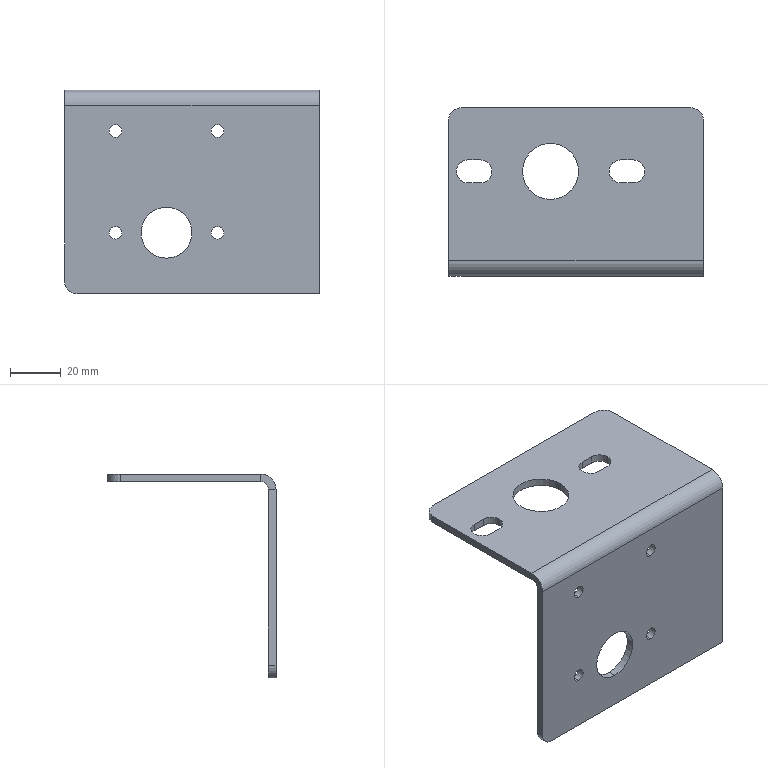Part | SolidWorks | features BaseBody 1 | 1 solid | 39 faces | box 100 x 66 x 80 mm | volume 39302 mm3 | cylinder 23 | plane 16 | commonest cylinder face diameters 5 x8 9 x6 10 x3 20 x2 22 x2 6 x1
STEP:
#1=CARTESIAN_POINT('',(-45.,-34.5,-77.));
#2=VERTEX_POINT('',#1);
#3=CARTESIAN_POINT('',(-50.,-34.5,-72.));
#4=VERTEX_POINT('',#3);
#5=CARTESIAN_POINT('',(-45.,-34.5,-72.));
#6=DIRECTION('',(0.,1.,0.));
#7=DIRECTION('',(0.,0.,1.));
#8=AXIS2_PLACEMENT_3D('',#5,#6,#7);
#9=CIRCLE('',#8,5.);
#10=EDGE_CURVE('',#2,#4,#9,.T.);
#11=ORIENTED_EDGE('',*,*,#10,.T.);
#12=CARTESIAN_POINT('',(-50.,-31.5,-72.));
#13=VERTEX_POINT('',#12);
#14=CARTESIAN_POINT('',(-50.,-34.5,-72.));
#15=DIRECTION('',(0.,1.,0.));
#16=VECTOR('',#15,1000.);
#17=LINE('',#14,#16);
#18=EDGE_CURVE('',#4,#13,#17,.T.);
#19=ORIENTED_EDGE('',*,*,#18,.T.);
#20=CARTESIAN_POINT('',(-45.,-31.5,-77.));
#21=VERTEX_POINT('',#20);
#22=CARTESIAN_POINT('',(-45.,-31.5,-72.));
#23=DIRECTION('',(0.,-1.,0.));
#24=DIRECTION('',(0.,0.,1.));
#25=AXIS2_PLACEMENT_3D('',#22,#23,#24);
#26=CIRCLE('',#25,5.);
#27=EDGE_CURVE('',#13,#21,#26,.T.);
#28=ORIENTED_EDGE('',*,*,#27,.T.);
#29=CARTESIAN_POINT('',(-45.,-34.5,-77.));
#30=DIRECTION('',(0.,-1.,0.));
#31=VECTOR('',#30,1000.);
#32=LINE('',#29,#31);
#33=EDGE_CURVE('',#21,#2,#32,.T.);
#34=ORIENTED_EDGE('',*,*,#33,.T.);
#35=EDGE_LOOP('',(#11,#19,#28,#34));
#36=FACE_OUTER_BOUND('',#35,.T.);
#37=CARTESIAN_POINT('',(-45.,-34.5,-72.));
#38=DIRECTION('',(0.,1.,0.));
#39=DIRECTION('',(0.,0.,-1.));
#40=AXIS2_PLACEMENT_3D('',#37,#38,#39);
#41=CYLINDRICAL_SURFACE('',#40,5.);
#42=ADVANCED_FACE('',(#36),#41,.T.);
#43=CARTESIAN_POINT('',(10.,-34.5,-50.5));
#44=VERTEX_POINT('',#43);
#45=CARTESIAN_POINT('',(10.,-31.5,-50.5));
#46=VERTEX_POINT('',#45);
#47=CARTESIAN_POINT('',(10.,-41.5,-50.5));
#48=DIRECTION('',(0.,1.,0.));
#49=VECTOR('',#48,1000.);
#50=LINE('',#47,#49);
#51=EDGE_CURVE('',#44,#46,#50,.T.);
#52=ORIENTED_EDGE('',*,*,#51,.F.);
#53=CARTESIAN_POINT('',(10.,-34.5,-55.5));
#54=VERTEX_POINT('',#53);
#55=CARTESIAN_POINT('',(10.,-34.5,-53.));
#56=DIRECTION('',(0.,1.,0.));
#57=DIRECTION('',(0.,0.,1.));
#58=AXIS2_PLACEMENT_3D('',#55,#56,#57);
#59=CIRCLE('',#58,2.5);
#60=EDGE_CURVE('',#54,#44,#59,.T.);
#61=ORIENTED_EDGE('',*,*,#60,.F.);
#62=CARTESIAN_POINT('',(10.,-31.5,-55.5));
#63=VERTEX_POINT('',#62);
#64=CARTESIAN_POINT('',(10.,-41.5,-55.5));
#65=DIRECTION('',(0.,1.,0.));
#66=VECTOR('',#65,1000.);
#67=LINE('',#64,#66);
#68=EDGE_CURVE('',#54,#63,#67,.T.);
#69=ORIENTED_EDGE('',*,*,#68,.T.);
#70=CARTESIAN_POINT('',(10.,-31.5,-53.));
#71=DIRECTION('',(0.,-1.,0.));
#72=DIRECTION('',(0.,0.,-1.));
#73=AXIS2_PLACEMENT_3D('',#70,#71,#72);
#74=CIRCLE('',#73,2.5);
#75=EDGE_CURVE('',#46,#63,#74,.T.);
#76=ORIENTED_EDGE('',*,*,#75,.F.);
#77=EDGE_LOOP('',(#52,#61,#69,#76));
#78=FACE_OUTER_BOUND('',#77,.T.);
#79=CARTESIAN_POINT('',(10.,-41.5,-53.));
#80=DIRECTION('',(0.,1.,0.));
#81=DIRECTION('',(0.,0.,-1.));
#82=AXIS2_PLACEMENT_3D('',#79,#80,#81);
#83=CYLINDRICAL_SURFACE('',#82,2.5);
#84=ADVANCED_FACE('',(#78),#83,.F.);
#85=CARTESIAN_POINT('',(10.,-34.5,-10.5));
#86=VERTEX_POINT('',#85);
#87=CARTESIAN_POINT('',(10.,-31.5,-10.5));
#88=VERTEX_POINT('',#87);
#89=CARTESIAN_POINT('',(10.,-41.5,-10.5));
#90=DIRECTION('',(0.,1.,0.));
#91=VECTOR('',#90,1000.);
#92=LINE('',#89,#91);
#93=EDGE_CURVE('',#86,#88,#92,.T.);
#94=ORIENTED_EDGE('',*,*,#93,.F.);
#95=CARTESIAN_POINT('',(10.,-34.5,-15.5));
#96=VERTEX_POINT('',#95);
#97=CARTESIAN_POINT('',(10.,-34.5,-13.));
#98=DIRECTION('',(0.,1.,0.));
#99=DIRECTION('',(0.,0.,1.));
#100=AXIS2_PLACEMENT_3D('',#97,#98,#99);
#101=CIRCLE('',#100,2.5);
#102=EDGE_CURVE('',#96,#86,#101,.T.);
#103=ORIENTED_EDGE('',*,*,#102,.F.);
#104=CARTESIAN_POINT('',(10.,-31.5,-15.5));
#105=VERTEX_POINT('',#104);
#106=CARTESIAN_POINT('',(10.,-41.5,-15.5));
#107=DIRECTION('',(0.,1.,0.));
#108=VECTOR('',#107,1000.);
#109=LINE('',#106,#108);
#110=EDGE_CURVE('',#96,#105,#109,.T.);
#111=ORIENTED_EDGE('',*,*,#110,.T.);
#112=CARTESIAN_POINT('',(10.,-31.5,-13.));
#113=DIRECTION('',(0.,-1.,0.));
#114=DIRECTION('',(0.,0.,-1.));
#115=AXIS2_PLACEMENT_3D('',#112,#113,#114);
#116=CIRCLE('',#115,2.5);
#117=EDGE_CURVE('',#88,#105,#116,.T.);
#118=ORIENTED_EDGE('',*,*,#117,.F.);
#119=EDGE_LOOP('',(#94,#103,#111,#118));
#120=FACE_OUTER_BOUND('',#119,.T.);
#121=CARTESIAN_POINT('',(10.,-41.5,-13.));
#122=DIRECTION('',(0.,1.,0.));
#123=DIRECTION('',(0.,0.,-1.));
#124=AXIS2_PLACEMENT_3D('',#121,#122,#123);
#125=CYLINDRICAL_SURFACE('',#124,2.5);
#126=ADVANCED_FACE('',(#120),#125,.F.);
#127=CARTESIAN_POINT('',(-30.,-34.5,-10.5));
#128=VERTEX_POINT('',#127);
#129=CARTESIAN_POINT('',(-30.,-31.5,-10.5));
#130=VERTEX_POINT('',#129);
#131=CARTESIAN_POINT('',(-30.,-41.5,-10.5));
#132=DIRECTION('',(0.,1.,0.));
#133=VECTOR('',#132,1000.);
#134=LINE('',#131,#133);
#135=EDGE_CURVE('',#128,#130,#134,.T.);
#136=ORIENTED_EDGE('',*,*,#135,.F.);
#137=CARTESIAN_POINT('',(-30.,-34.5,-15.5));
#138=VERTEX_POINT('',#137);
#139=CARTESIAN_POINT('',(-30.,-34.5,-13.));
#140=DIRECTION('',(0.,1.,0.));
#141=DIRECTION('',(0.,0.,1.));
#142=AXIS2_PLACEMENT_3D('',#139,#140,#141);
#143=CIRCLE('',#142,2.5);
#144=EDGE_CURVE('',#138,#128,#143,.T.);
#145=ORIENTED_EDGE('',*,*,#144,.F.);
#146=CARTESIAN_POINT('',(-30.,-31.5,-15.5));
#147=VERTEX_POINT('',#146);
#148=CARTESIAN_POINT('',(-30.,-41.5,-15.5));
#149=DIRECTION('',(0.,1.,0.));
#150=VECTOR('',#149,1000.);
#151=LINE('',#148,#150);
#152=EDGE_CURVE('',#138,#147,#151,.T.);
#153=ORIENTED_EDGE('',*,*,#152,.T.);
#154=CARTESIAN_POINT('',(-30.,-31.5,-13.));
#155=DIRECTION('',(0.,-1.,0.));
#156=DIRECTION('',(0.,0.,-1.));
#157=AXIS2_PLACEMENT_3D('',#154,#155,#156);
#158=CIRCLE('',#157,2.5);
#159=EDGE_CURVE('',#130,#147,#158,.T.);
#160=ORIENTED_EDGE('',*,*,#159,.F.);
#161=EDGE_LOOP('',(#136,#145,#153,#160));
#162=FACE_OUTER_BOUND('',#161,.T.);
#163=CARTESIAN_POINT('',(-30.,-41.5,-13.));
#164=DIRECTION('',(0.,1.,0.));
#165=DIRECTION('',(0.,0.,-1.));
#166=AXIS2_PLACEMENT_3D('',#163,#164,#165);
#167=CYLINDRICAL_SURFACE('',#166,2.5);
#168=ADVANCED_FACE('',(#162),#167,.F.);
#169=CARTESIAN_POINT('',(-30.,-34.5,-50.5));
#170=VERTEX_POINT('',#169);
#171=CARTESIAN_POINT('',(-30.,-31.5,-50.5));
#172=VERTEX_POINT('',#171);
#173=CARTESIAN_POINT('',(-30.,-41.5,-50.5));
#174=DIRECTION('',(0.,1.,0.));
#175=VECTOR('',#174,1000.);
#176=LINE('',#173,#175);
#177=EDGE_CURVE('',#170,#172,#176,.T.);
#178=ORIENTED_EDGE('',*,*,#177,.F.);
#179=CARTESIAN_POINT('',(-30.,-34.5,-55.5));
#180=VERTEX_POINT('',#179);
#181=CARTESIAN_POINT('',(-30.,-34.5,-53.));
#182=DIRECTION('',(0.,1.,0.));
#183=DIRECTION('',(0.,0.,1.));
#184=AXIS2_PLACEMENT_3D('',#181,#182,#183);
#185=CIRCLE('',#184,2.5);
#186=EDGE_CURVE('',#180,#170,#185,.T.);
#187=ORIENTED_EDGE('',*,*,#186,.F.);
#188=CARTESIAN_POINT('',(-30.,-31.5,-55.5));
#189=VERTEX_POINT('',#188);
#190=CARTESIAN_POINT('',(-30.,-41.5,-55.5));
#191=DIRECTION('',(0.,1.,0.));
#192=VECTOR('',#191,1000.);
#193=LINE('',#190,#192);
#194=EDGE_CURVE('',#180,#189,#193,.T.);
#195=ORIENTED_EDGE('',*,*,#194,.T.);
#196=CARTESIAN_POINT('',(-30.,-31.5,-53.));
#197=DIRECTION('',(0.,-1.,0.));
#198=DIRECTION('',(0.,0.,-1.));
#199=AXIS2_PLACEMENT_3D('',#196,#197,#198);
#200=CIRCLE('',#199,2.5);
#201=EDGE_CURVE('',#172,#189,#200,.T.);
#202=ORIENTED_EDGE('',*,*,#201,.F.);
#203=EDGE_LOOP('',(#178,#187,#195,#202));
#204=FACE_OUTER_BOUND('',#203,.T.);
#205=CARTESIAN_POINT('',(-30.,-41.5,-53.));
#206=DIRECTION('',(0.,1.,0.));
#207=DIRECTION('',(0.,0.,-1.));
#208=AXIS2_PLACEMENT_3D('',#205,#206,#207);
#209=CYLINDRICAL_SURFACE('',#208,2.5);
#210=ADVANCED_FACE('',(#204),#209,.F.);
#211=CARTESIAN_POINT('',(-10.,-34.5,-43.));
#212=VERTEX_POINT('',#211);
#213=CARTESIAN_POINT('',(-10.,-31.5,-43.));
#214=VERTEX_POINT('',#213);
#215=CARTESIAN_POINT('',(-10.,-41.5,-43.));
#216=DIRECTION('',(0.,1.,0.));
#217=VECTOR('',#216,1000.);
#218=LINE('',#215,#217);
#219=EDGE_CURVE('',#212,#214,#218,.T.);
#220=ORIENTED_EDGE('',*,*,#219,.F.);
#221=CARTESIAN_POINT('',(-10.,-34.5,-63.));
#222=VERTEX_POINT('',#221);
#223=CARTESIAN_POINT('',(-10.,-34.5,-53.));
#224=DIRECTION('',(0.,1.,0.));
#225=DIRECTION('',(0.,0.,1.));
#226=AXIS2_PLACEMENT_3D('',#223,#224,#225);
#227=CIRCLE('',#226,10.);
#228=EDGE_CURVE('',#222,#212,#227,.T.);
#229=ORIENTED_EDGE('',*,*,#228,.F.);
#230=CARTESIAN_POINT('',(-10.,-31.5,-63.));
#231=VERTEX_POINT('',#230);
#232=CARTESIAN_POINT('',(-10.,-41.5,-63.));
#233=DIRECTION('',(0.,1.,0.));
#234=VECTOR('',#233,1000.);
#235=LINE('',#232,#234);
#236=EDGE_CURVE('',#222,#231,#235,.T.);
#237=ORIENTED_EDGE('',*,*,#236,.T.);
#238=CARTESIAN_POINT('',(-10.,-31.5,-53.));
#239=DIRECTION('',(0.,-1.,0.));
#240=DIRECTION('',(0.,0.,-1.));
#241=AXIS2_PLACEMENT_3D('',#238,#239,#240);
#242=CIRCLE('',#241,10.);
#243=EDGE_CURVE('',#214,#231,#242,.T.);
#244=ORIENTED_EDGE('',*,*,#243,.F.);
#245=EDGE_LOOP('',(#220,#229,#237,#244));
#246=FACE_OUTER_BOUND('',#245,.T.);
#247=CARTESIAN_POINT('',(-10.,-41.5,-53.));
#248=DIRECTION('',(0.,1.,0.));
#249=DIRECTION('',(0.,0.,-1.));
#250=AXIS2_PLACEMENT_3D('',#247,#248,#249);
#251=CYLINDRICAL_SURFACE('',#250,10.);
#252=ADVANCED_FACE('',(#246),#251,.F.);
#253=CARTESIAN_POINT('',(-50.,26.5,3.));
#254=VERTEX_POINT('',#253);
#255=CARTESIAN_POINT('',(-45.,31.5,3.));
#256=VERTEX_POINT('',#255);
#257=CARTESIAN_POINT('',(-45.,26.5,3.));
#258=DIRECTION('',(0.,0.,-1.));
#259=DIRECTION('',(1.,0.,0.));
#260=AXIS2_PLACEMENT_3D('',#257,#258,#259);
#261=CIRCLE('',#260,5.);
#262=EDGE_CURVE('',#254,#256,#261,.T.);
#263=ORIENTED_EDGE('',*,*,#262,.T.);
#264=CARTESIAN_POINT('',(-45.,31.5,0.));
#265=VERTEX_POINT('',#264);
#266=CARTESIAN_POINT('',(-45.,31.5,3.));
#267=DIRECTION('',(0.,0.,-1.));
#268=VECTOR('',#267,1000.);
#269=LINE('',#266,#268);
#270=EDGE_CURVE('',#256,#265,#269,.T.);
#271=ORIENTED_EDGE('',*,*,#270,.T.);
#272=CARTESIAN_POINT('',(-50.,26.5,0.));
#273=VERTEX_POINT('',#272);
#274=CARTESIAN_POINT('',(-45.,26.5,0.));
#275=DIRECTION('',(0.,0.,1.));
#276=DIRECTION('',(1.,0.,0.));
#277=AXIS2_PLACEMENT_3D('',#274,#275,#276);
#278=CIRCLE('',#277,5.);
#279=EDGE_CURVE('',#265,#273,#278,.T.);
#280=ORIENTED_EDGE('',*,*,#279,.T.);
#281=CARTESIAN_POINT('',(-50.,26.5,3.));
#282=DIRECTION('',(0.,0.,1.));
#283=VECTOR('',#282,1000.);
#284=LINE('',#281,#283);
#285=EDGE_CURVE('',#273,#254,#284,.T.);
#286=ORIENTED_EDGE('',*,*,#285,.T.);
#287=EDGE_LOOP('',(#263,#271,#280,#286));
#288=FACE_OUTER_BOUND('',#287,.T.);
#289=CARTESIAN_POINT('',(-45.,26.5,3.));
#290=DIRECTION('',(0.,0.,-1.));
#291=DIRECTION('',(1.,0.,0.));
#292=AXIS2_PLACEMENT_3D('',#289,#290,#291);
#293=CYLINDRICAL_SURFACE('',#292,5.);
#294=ADVANCED_FACE('',(#288),#293,.T.);
#295=CARTESIAN_POINT('',(45.,31.5,3.));
#296=VERTEX_POINT('',#295);
#297=CARTESIAN_POINT('',(50.,26.5,3.));
#298=VERTEX_POINT('',#297);
#299=CARTESIAN_POINT('',(45.,26.5,3.));
#300=DIRECTION('',(0.,0.,-1.));
#301=DIRECTION('',(1.,0.,0.));
#302=AXIS2_PLACEMENT_3D('',#299,#300,#301);
#303=CIRCLE('',#302,5.);
#304=EDGE_CURVE('',#296,#298,#303,.T.);
#305=ORIENTED_EDGE('',*,*,#304,.T.);
#306=CARTESIAN_POINT('',(50.,26.5,0.));
#307=VERTEX_POINT('',#306);
#308=CARTESIAN_POINT('',(50.,26.5,3.));
#309=DIRECTION('',(0.,0.,-1.));
#310=VECTOR('',#309,1000.);
#311=LINE('',#308,#310);
#312=EDGE_CURVE('',#298,#307,#311,.T.);
#313=ORIENTED_EDGE('',*,*,#312,.T.);
#314=CARTESIAN_POINT('',(45.,31.5,0.));
#315=VERTEX_POINT('',#314);
#316=CARTESIAN_POINT('',(45.,26.5,0.));
#317=DIRECTION('',(0.,0.,1.));
#318=DIRECTION('',(1.,0.,0.));
#319=AXIS2_PLACEMENT_3D('',#316,#317,#318);
#320=CIRCLE('',#319,5.);
#321=EDGE_CURVE('',#307,#315,#320,.T.);
#322=ORIENTED_EDGE('',*,*,#321,.T.);
#323=CARTESIAN_POINT('',(45.,31.5,3.));
#324=DIRECTION('',(0.,0.,1.));
#325=VECTOR('',#324,1000.);
#326=LINE('',#323,#325);
#327=EDGE_CURVE('',#315,#296,#326,.T.);
#328=ORIENTED_EDGE('',*,*,#327,.T.);
#329=EDGE_LOOP('',(#305,#313,#322,#328));
#330=FACE_OUTER_BOUND('',#329,.T.);
#331=CARTESIAN_POINT('',(45.,26.5,3.));
#332=DIRECTION('',(0.,0.,-1.));
#333=DIRECTION('',(1.,0.,0.));
#334=AXIS2_PLACEMENT_3D('',#331,#332,#333);
#335=CYLINDRICAL_SURFACE('',#334,5.);
#336=ADVANCED_FACE('',(#330),#335,.T.);
#337=CARTESIAN_POINT('',(50.,-31.5,-77.));
#338=VERTEX_POINT('',#337);
#339=CARTESIAN_POINT('',(50.,-31.5,-77.));
#340=DIRECTION('',(1.,0.,0.));
#341=VECTOR('',#340,1000.);
#342=LINE('',#339,#341);
#343=EDGE_CURVE('',#21,#338,#342,.T.);
#344=ORIENTED_EDGE('',*,*,#343,.T.);
#345=CARTESIAN_POINT('',(50.,-34.5,-77.));
#346=VERTEX_POINT('',#345);
#347=CARTESIAN_POINT('',(50.,-34.5,-77.));
#348=DIRECTION('',(0.,1.,0.));
#349=VECTOR('',#348,1000.);
#350=LINE('',#347,#349);
#351=EDGE_CURVE('',#346,#338,#350,.T.);
#352=ORIENTED_EDGE('',*,*,#351,.F.);
#353=CARTESIAN_POINT('',(50.,-34.5,-77.));
#354=DIRECTION('',(1.,0.,0.));
#355=VECTOR('',#354,1000.);
#356=LINE('',#353,#355);
#357=EDGE_CURVE('',#2,#346,#356,.T.);
#358=ORIENTED_EDGE('',*,*,#357,.F.);
#359=ORIENTED_EDGE('',*,*,#33,.F.);
#360=EDGE_LOOP('',(#344,#352,#358,#359));
#361=FACE_OUTER_BOUND('',#360,.T.);
#362=CARTESIAN_POINT('',(50.,-34.5,-77.));
#363=DIRECTION('',(0.,0.,-1.));
#364=DIRECTION('',(0.,-1.,0.));
#365=AXIS2_PLACEMENT_3D('',#362,#363,#364);
#366=PLANE('',#365);
#367=ADVANCED_FACE('',(#361),#366,.T.);
#368=CARTESIAN_POINT('',(-10.,-31.5,-53.));
#369=DIRECTION('',(0.,-1.,0.));
#370=DIRECTION('',(0.,0.,-1.));
#371=AXIS2_PLACEMENT_3D('',#368,#369,#370);
#372=CIRCLE('',#371,10.);
#373=EDGE_CURVE('',#231,#214,#372,.T.);
#374=ORIENTED_EDGE('',*,*,#373,.T.);
#375=ORIENTED_EDGE('',*,*,#243,.T.);
#376=EDGE_LOOP('',(#374,#375));
#377=FACE_BOUND('',#376,.T.);
#378=CARTESIAN_POINT('',(-30.,-31.5,-53.));
#379=DIRECTION('',(0.,-1.,0.));
#380=DIRECTION('',(0.,0.,-1.));
#381=AXIS2_PLACEMENT_3D('',#378,#379,#380);
#382=CIRCLE('',#381,2.5);
#383=EDGE_CURVE('',#189,#172,#382,.T.);
#384=ORIENTED_EDGE('',*,*,#383,.T.);
#385=ORIENTED_EDGE('',*,*,#201,.T.);
#386=EDGE_LOOP('',(#384,#385));
#387=FACE_BOUND('',#386,.T.);
#388=CARTESIAN_POINT('',(-30.,-31.5,-13.));
#389=DIRECTION('',(0.,-1.,0.));
#390=DIRECTION('',(0.,0.,-1.));
#391=AXIS2_PLACEMENT_3D('',#388,#389,#390);
#392=CIRCLE('',#391,2.5);
#393=EDGE_CURVE('',#147,#130,#392,.T.);
#394=ORIENTED_EDGE('',*,*,#393,.T.);
#395=ORIENTED_EDGE('',*,*,#159,.T.);
#396=EDGE_LOOP('',(#394,#395));
#397=FACE_BOUND('',#396,.T.);
#398=CARTESIAN_POINT('',(10.,-31.5,-13.));
#399=DIRECTION('',(0.,-1.,0.));
#400=DIRECTION('',(0.,0.,-1.));
#401=AXIS2_PLACEMENT_3D('',#398,#399,#400);
#402=CIRCLE('',#401,2.5);
#403=EDGE_CURVE('',#105,#88,#402,.T.);
#404=ORIENTED_EDGE('',*,*,#403,.T.);
#405=ORIENTED_EDGE('',*,*,#117,.T.);
#406=EDGE_LOOP('',(#404,#405));
#407=FACE_BOUND('',#406,.T.);
#408=CARTESIAN_POINT('',(10.,-31.5,-53.));
#409=DIRECTION('',(0.,-1.,0.));
#410=DIRECTION('',(0.,0.,-1.));
#411=AXIS2_PLACEMENT_3D('',#408,#409,#410);
#412=CIRCLE('',#411,2.5);
#413=EDGE_CURVE('',#63,#46,#412,.T.);
#414=ORIENTED_EDGE('',*,*,#413,.T.);
#415=ORIENTED_EDGE('',*,*,#75,.T.);
#416=EDGE_LOOP('',(#414,#415));
#417=FACE_BOUND('',#416,.T.);
#418=CARTESIAN_POINT('',(-50.,-31.5,-3.));
#419=VERTEX_POINT('',#418);
#420=CARTESIAN_POINT('',(-50.,-31.5,-77.));
#421=DIRECTION('',(0.,0.,-1.));
#422=VECTOR('',#421,1000.);
#423=LINE('',#420,#422);
#424=EDGE_CURVE('',#419,#13,#423,.T.);
#425=ORIENTED_EDGE('',*,*,#424,.F.);
#426=CARTESIAN_POINT('',(50.,-31.5,-3.));
#427=VERTEX_POINT('',#426);
#428=CARTESIAN_POINT('',(-50.,-31.5,-3.));
#429=DIRECTION('',(1.,0.,0.));
#430=VECTOR('',#429,1000.);
#431=LINE('',#428,#430);
#432=EDGE_CURVE('',#419,#427,#431,.T.);
#433=ORIENTED_EDGE('',*,*,#432,.T.);
#434=CARTESIAN_POINT('',(50.,-31.5,0.));
#435=DIRECTION('',(0.,0.,1.));
#436=VECTOR('',#435,1000.);
#437=LINE('',#434,#436);
#438=EDGE_CURVE('',#338,#427,#437,.T.);
#439=ORIENTED_EDGE('',*,*,#438,.F.);
#440=ORIENTED_EDGE('',*,*,#343,.F.);
#441=ORIENTED_EDGE('',*,*,#27,.F.);
#442=EDGE_LOOP('',(#425,#433,#439,#440,#441));
#443=FACE_OUTER_BOUND('',#442,.T.);
#444=CARTESIAN_POINT('',(0.,-31.5,0.));
#445=DIRECTION('',(0.,-1.,0.));
#446=DIRECTION('',(-1.,0.,0.));
#447=AXIS2_PLACEMENT_3D('',#444,#445,#446);
#448=PLANE('',#447);
#449=ADVANCED_FACE('',(#377,#387,#397,#407,#417,#443),#448,.F.);
#450=ORIENTED_EDGE('',*,*,#228,.T.);
#451=CARTESIAN_POINT('',(-10.,-34.5,-53.));
#452=DIRECTION('',(0.,1.,0.));
#453=DIRECTION('',(0.,0.,1.));
#454=AXIS2_PLACEMENT_3D('',#451,#452,#453);
#455=CIRCLE('',#454,10.);
#456=EDGE_CURVE('',#212,#222,#455,.T.);
#457=ORIENTED_EDGE('',*,*,#456,.T.);
#458=EDGE_LOOP('',(#450,#457));
#459=FACE_BOUND('',#458,.T.);
#460=ORIENTED_EDGE('',*,*,#186,.T.);
#461=CARTESIAN_POINT('',(-30.,-34.5,-53.));
#462=DIRECTION('',(0.,1.,0.));
#463=DIRECTION('',(0.,0.,1.));
#464=AXIS2_PLACEMENT_3D('',#461,#462,#463);
#465=CIRCLE('',#464,2.5);
#466=EDGE_CURVE('',#170,#180,#465,.T.);
#467=ORIENTED_EDGE('',*,*,#466,.T.);
#468=EDGE_LOOP('',(#460,#467));
#469=FACE_BOUND('',#468,.T.);
#470=ORIENTED_EDGE('',*,*,#144,.T.);
#471=CARTESIAN_POINT('',(-30.,-34.5,-13.));
#472=DIRECTION('',(0.,1.,0.));
#473=DIRECTION('',(0.,0.,1.));
#474=AXIS2_PLACEMENT_3D('',#471,#472,#473);
#475=CIRCLE('',#474,2.5);
#476=EDGE_CURVE('',#128,#138,#475,.T.);
#477=ORIENTED_EDGE('',*,*,#476,.T.);
#478=EDGE_LOOP('',(#470,#477));
#479=FACE_BOUND('',#478,.T.);
#480=ORIENTED_EDGE('',*,*,#102,.T.);
#481=CARTESIAN_POINT('',(10.,-34.5,-13.));
#482=DIRECTION('',(0.,1.,0.));
#483=DIRECTION('',(0.,0.,1.));
#484=AXIS2_PLACEMENT_3D('',#481,#482,#483);
#485=CIRCLE('',#484,2.5);
#486=EDGE_CURVE('',#86,#96,#485,.T.);
#487=ORIENTED_EDGE('',*,*,#486,.T.);
#488=EDGE_LOOP('',(#480,#487));
#489=FACE_BOUND('',#488,.T.);
#490=ORIENTED_EDGE('',*,*,#60,.T.);
#491=CARTESIAN_POINT('',(10.,-34.5,-53.));
#492=DIRECTION('',(0.,1.,0.));
#493=DIRECTION('',(0.,0.,1.));
#494=AXIS2_PLACEMENT_3D('',#491,#492,#493);
#495=CIRCLE('',#494,2.5);
#496=EDGE_CURVE('',#44,#54,#495,.T.);
#497=ORIENTED_EDGE('',*,*,#496,.T.);
#498=EDGE_LOOP('',(#490,#497));
#499=FACE_BOUND('',#498,.T.);
#500=ORIENTED_EDGE('',*,*,#357,.T.);
#501=CARTESIAN_POINT('',(50.,-34.5,-3.));
#502=VERTEX_POINT('',#501);
#503=CARTESIAN_POINT('',(50.,-34.5,0.));
#504=DIRECTION('',(0.,0.,1.));
#505=VECTOR('',#504,1000.);
#506=LINE('',#503,#505);
#507=EDGE_CURVE('',#346,#502,#506,.T.);
#508=ORIENTED_EDGE('',*,*,#507,.T.);
#509=CARTESIAN_POINT('',(-50.,-34.5,-3.));
#510=VERTEX_POINT('',#509);
#511=CARTESIAN_POINT('',(0.,-34.5,-3.));
#512=DIRECTION('',(1.,0.,0.));
#513=VECTOR('',#512,1000.);
#514=LINE('',#511,#513);
#515=EDGE_CURVE('',#510,#502,#514,.T.);
#516=ORIENTED_EDGE('',*,*,#515,.F.);
#517=CARTESIAN_POINT('',(-50.,-34.5,-77.));
#518=DIRECTION('',(0.,0.,-1.));
#519=VECTOR('',#518,1000.);
#520=LINE('',#517,#519);
#521=EDGE_CURVE('',#510,#4,#520,.T.);
#522=ORIENTED_EDGE('',*,*,#521,.T.);
#523=ORIENTED_EDGE('',*,*,#10,.F.);
#524=EDGE_LOOP('',(#500,#508,#516,#522,#523));
#525=FACE_OUTER_BOUND('',#524,.T.);
#526=CARTESIAN_POINT('',(0.,-34.5,0.));
#527=DIRECTION('',(0.,-1.,0.));
#528=DIRECTION('',(-1.,0.,0.));
#529=AXIS2_PLACEMENT_3D('',#526,#527,#528);
#530=PLANE('',#529);
#531=ADVANCED_FACE('',(#459,#469,#479,#489,#499,#525),#530,.T.);
#532=ORIENTED_EDGE('',*,*,#521,.F.);
#533=CARTESIAN_POINT('',(-50.,-31.5,-3.));
#534=DIRECTION('',(0.,-1.,0.));
#535=VECTOR('',#534,1000.);
#536=LINE('',#533,#535);
#537=EDGE_CURVE('',#419,#510,#536,.T.);
#538=ORIENTED_EDGE('',*,*,#537,.F.);
#539=ORIENTED_EDGE('',*,*,#424,.T.);
#540=ORIENTED_EDGE('',*,*,#18,.F.);
#541=EDGE_LOOP('',(#532,#538,#539,#540));
#542=FACE_OUTER_BOUND('',#541,.T.);
#543=CARTESIAN_POINT('',(-50.,-34.5,-77.));
#544=DIRECTION('',(-1.,0.,0.));
#545=DIRECTION('',(0.,0.,1.));
#546=AXIS2_PLACEMENT_3D('',#543,#544,#545);
#547=PLANE('',#546);
#548=ADVANCED_FACE('',(#542),#547,.T.);
#549=ORIENTED_EDGE('',*,*,#507,.F.);
#550=ORIENTED_EDGE('',*,*,#351,.T.);
#551=ORIENTED_EDGE('',*,*,#438,.T.);
#552=CARTESIAN_POINT('',(50.,-31.5,-3.));
#553=DIRECTION('',(0.,-1.,0.));
#554=VECTOR('',#553,1000.);
#555=LINE('',#552,#554);
#556=EDGE_CURVE('',#427,#502,#555,.T.);
#557=ORIENTED_EDGE('',*,*,#556,.T.);
#558=EDGE_LOOP('',(#549,#550,#551,#557));
#559=FACE_OUTER_BOUND('',#558,.T.);
#560=CARTESIAN_POINT('',(50.,-34.5,0.));
#561=DIRECTION('',(1.,0.,0.));
#562=DIRECTION('',(0.,1.,0.));
#563=AXIS2_PLACEMENT_3D('',#560,#561,#562);
#564=PLANE('',#563);
#565=ADVANCED_FACE('',(#559),#564,.T.);
#566=CARTESIAN_POINT('',(50.,-28.5,0.));
#567=VERTEX_POINT('',#566);
#568=CARTESIAN_POINT('',(-50.,-28.5,0.));
#569=VERTEX_POINT('',#568);
#570=CARTESIAN_POINT('',(50.,-28.5,0.));
#571=DIRECTION('',(-1.,0.,0.));
#572=VECTOR('',#571,1000.);
#573=LINE('',#570,#572);
#574=EDGE_CURVE('',#567,#569,#573,.T.);
#575=ORIENTED_EDGE('',*,*,#574,.F.);
#576=CARTESIAN_POINT('',(50.,-28.5,-3.));
#577=DIRECTION('',(-1.,0.,0.));
#578=DIRECTION('',(0.,0.,1.));
#579=AXIS2_PLACEMENT_3D('',#576,#577,#578);
#580=CIRCLE('',#579,3.);
#581=EDGE_CURVE('',#427,#567,#580,.T.);
#582=ORIENTED_EDGE('',*,*,#581,.F.);
#583=ORIENTED_EDGE('',*,*,#432,.F.);
#584=CARTESIAN_POINT('',(-50.,-28.5,-3.));
#585=DIRECTION('',(1.,0.,0.));
#586=DIRECTION('',(0.,0.,1.));
#587=AXIS2_PLACEMENT_3D('',#584,#585,#586);
#588=CIRCLE('',#587,3.);
#589=EDGE_CURVE('',#569,#419,#588,.T.);
#590=ORIENTED_EDGE('',*,*,#589,.F.);
#591=EDGE_LOOP('',(#575,#582,#583,#590));
#592=FACE_OUTER_BOUND('',#591,.T.);
#593=CARTESIAN_POINT('',(50.,-28.5,-3.));
#594=DIRECTION('',(1.,0.,0.));
#595=DIRECTION('',(0.,-1.,0.));
#596=AXIS2_PLACEMENT_3D('',#593,#594,#595);
#597=CYLINDRICAL_SURFACE('',#596,3.);
#598=ADVANCED_FACE('',(#592),#597,.F.);
#599=CARTESIAN_POINT('',(50.,-28.5,3.));
#600=VERTEX_POINT('',#599);
#601=CARTESIAN_POINT('',(-50.,-28.5,3.));
#602=VERTEX_POINT('',#601);
#603=CARTESIAN_POINT('',(50.,-28.5,3.));
#604=DIRECTION('',(-1.,0.,0.));
#605=VECTOR('',#604,1000.);
#606=LINE('',#603,#605);
#607=EDGE_CURVE('',#600,#602,#606,.T.);
#608=ORIENTED_EDGE('',*,*,#607,.T.);
#609=CARTESIAN_POINT('',(-50.,-28.5,-3.));
#610=DIRECTION('',(1.,0.,0.));
#611=DIRECTION('',(0.,0.,1.));
#612=AXIS2_PLACEMENT_3D('',#609,#610,#611);
#613=CIRCLE('',#612,6.);
#614=EDGE_CURVE('',#602,#510,#613,.T.);
#615=ORIENTED_EDGE('',*,*,#614,.T.);
#616=ORIENTED_EDGE('',*,*,#515,.T.);
#617=CARTESIAN_POINT('',(50.,-28.5,-3.));
#618=DIRECTION('',(-1.,0.,0.));
#619=DIRECTION('',(0.,0.,1.));
#620=AXIS2_PLACEMENT_3D('',#617,#618,#619);
#621=CIRCLE('',#620,6.);
#622=EDGE_CURVE('',#502,#600,#621,.T.);
#623=ORIENTED_EDGE('',*,*,#622,.T.);
#624=EDGE_LOOP('',(#608,#615,#616,#623));
#625=FACE_OUTER_BOUND('',#624,.T.);
#626=CARTESIAN_POINT('',(50.,-28.5,-3.));
#627=DIRECTION('',(1.,0.,0.));
#628=DIRECTION('',(0.,-1.,0.));
#629=AXIS2_PLACEMENT_3D('',#626,#627,#628);
#630=CYLINDRICAL_SURFACE('',#629,6.);
#631=ADVANCED_FACE('',(#625),#630,.T.);
#632=ORIENTED_EDGE('',*,*,#581,.T.);
#633=CARTESIAN_POINT('',(50.,-28.5,0.));
#634=DIRECTION('',(0.,0.,1.));
#635=VECTOR('',#634,1000.);
#636=LINE('',#633,#635);
#637=EDGE_CURVE('',#567,#600,#636,.T.);
#638=ORIENTED_EDGE('',*,*,#637,.T.);
#639=ORIENTED_EDGE('',*,*,#622,.F.);
#640=ORIENTED_EDGE('',*,*,#556,.F.);
#641=EDGE_LOOP('',(#632,#638,#639,#640));
#642=FACE_OUTER_BOUND('',#641,.T.);
#643=CARTESIAN_POINT('',(50.,-28.5,-3.));
#644=DIRECTION('',(-1.,0.,0.));
#645=DIRECTION('',(0.,0.,1.));
#646=AXIS2_PLACEMENT_3D('',#643,#644,#645);
#647=PLANE('',#646);
#648=ADVANCED_FACE('',(#642),#647,.F.);
#649=ORIENTED_EDGE('',*,*,#537,.T.);
#650=ORIENTED_EDGE('',*,*,#614,.F.);
#651=CARTESIAN_POINT('',(-50.,-28.5,0.));
#652=DIRECTION('',(0.,0.,1.));
#653=VECTOR('',#652,1000.);
#654=LINE('',#651,#653);
#655=EDGE_CURVE('',#569,#602,#654,.T.);
#656=ORIENTED_EDGE('',*,*,#655,.F.);
#657=ORIENTED_EDGE('',*,*,#589,.T.);
#658=EDGE_LOOP('',(#649,#650,#656,#657));
#659=FACE_OUTER_BOUND('',#658,.T.);
#660=CARTESIAN_POINT('',(-50.,-28.5,-3.));
#661=DIRECTION('',(-1.,0.,0.));
#662=DIRECTION('',(0.,0.,1.));
#663=AXIS2_PLACEMENT_3D('',#660,#661,#662);
#664=PLANE('',#663);
#665=ADVANCED_FACE('',(#659),#664,.T.);
#666=CARTESIAN_POINT('',(-42.5,2.,3.));
#667=VERTEX_POINT('',#666);
#668=CARTESIAN_POINT('',(-42.5,2.,0.));
#669=VERTEX_POINT('',#668);
#670=CARTESIAN_POINT('',(-42.5,2.,10.));
#671=DIRECTION('',(0.,0.,-1.));
#672=VECTOR('',#671,1000.);
#673=LINE('',#670,#672);
#674=EDGE_CURVE('',#667,#669,#673,.T.);
#675=ORIENTED_EDGE('',*,*,#674,.F.);
#676=CARTESIAN_POINT('',(-37.5,2.,3.));
#677=VERTEX_POINT('',#676);
#678=CARTESIAN_POINT('',(0.,2.,3.));
#679=DIRECTION('',(1.,0.,0.));
#680=VECTOR('',#679,1000.);
#681=LINE('',#678,#680);
#682=EDGE_CURVE('',#667,#677,#681,.T.);
#683=ORIENTED_EDGE('',*,*,#682,.T.);
#684=CARTESIAN_POINT('',(-37.5,2.,0.));
#685=VERTEX_POINT('',#684);
#686=CARTESIAN_POINT('',(-37.5,2.,10.));
#687=DIRECTION('',(0.,0.,-1.));
#688=VECTOR('',#687,1000.);
#689=LINE('',#686,#688);
#690=EDGE_CURVE('',#677,#685,#689,.T.);
#691=ORIENTED_EDGE('',*,*,#690,.T.);
#692=CARTESIAN_POINT('',(-42.5,2.,0.));
#693=DIRECTION('',(1.,0.,0.));
#694=VECTOR('',#693,1000.);
#695=LINE('',#692,#694);
#696=EDGE_CURVE('',#669,#685,#695,.T.);
#697=ORIENTED_EDGE('',*,*,#696,.F.);
#698=EDGE_LOOP('',(#675,#683,#691,#697));
#699=FACE_OUTER_BOUND('',#698,.T.);
#700=CARTESIAN_POINT('',(-42.5,2.,10.));
#701=DIRECTION('',(0.,-1.,0.));
#702=DIRECTION('',(0.,0.,-1.));
#703=AXIS2_PLACEMENT_3D('',#700,#701,#702);
#704=PLANE('',#703);
#705=ADVANCED_FACE('',(#699),#704,.F.);
#706=CARTESIAN_POINT('',(-33.,6.5,3.));
#707=VERTEX_POINT('',#706);
#708=CARTESIAN_POINT('',(-33.,6.5,0.));
#709=VERTEX_POINT('',#708);
#710=CARTESIAN_POINT('',(-33.,6.5,10.));
#711=DIRECTION('',(0.,0.,-1.));
#712=VECTOR('',#711,1000.);
#713=LINE('',#710,#712);
#714=EDGE_CURVE('',#707,#709,#713,.T.);
#715=ORIENTED_EDGE('',*,*,#714,.F.);
#716=CARTESIAN_POINT('',(-37.5,11.,3.));
#717=VERTEX_POINT('',#716);
#718=CARTESIAN_POINT('',(-37.5,6.5,3.));
#719=DIRECTION('',(0.,0.,1.));
#720=DIRECTION('',(1.,0.,0.));
#721=AXIS2_PLACEMENT_3D('',#718,#719,#720);
#722=CIRCLE('',#721,4.5);
#723=EDGE_CURVE('',#707,#717,#722,.T.);
#724=ORIENTED_EDGE('',*,*,#723,.T.);
#725=CARTESIAN_POINT('',(-37.5,11.,0.));
#726=VERTEX_POINT('',#725);
#727=CARTESIAN_POINT('',(-37.5,11.,10.));
#728=DIRECTION('',(0.,0.,-1.));
#729=VECTOR('',#728,1000.);
#730=LINE('',#727,#729);
#731=EDGE_CURVE('',#717,#726,#730,.T.);
#732=ORIENTED_EDGE('',*,*,#731,.T.);
#733=CARTESIAN_POINT('',(-37.5,6.5,0.));
#734=DIRECTION('',(0.,0.,1.));
#735=DIRECTION('',(1.,0.,0.));
#736=AXIS2_PLACEMENT_3D('',#733,#734,#735);
#737=CIRCLE('',#736,4.5);
#738=EDGE_CURVE('',#709,#726,#737,.T.);
#739=ORIENTED_EDGE('',*,*,#738,.F.);
#740=EDGE_LOOP('',(#715,#724,#732,#739));
#741=FACE_OUTER_BOUND('',#740,.T.);
#742=CARTESIAN_POINT('',(-37.5,6.5,10.));
#743=DIRECTION('',(0.,0.,-1.));
#744=DIRECTION('',(1.,0.,0.));
#745=AXIS2_PLACEMENT_3D('',#742,#743,#744);
#746=CYLINDRICAL_SURFACE('',#745,4.5);
#747=ADVANCED_FACE('',(#741),#746,.F.);
#748=ORIENTED_EDGE('',*,*,#731,.F.);
#749=CARTESIAN_POINT('',(-42.5,11.,3.));
#750=VERTEX_POINT('',#749);
#751=CARTESIAN_POINT('',(0.,11.,3.));
#752=DIRECTION('',(-1.,0.,0.));
#753=VECTOR('',#752,1000.);
#754=LINE('',#751,#753);
#755=EDGE_CURVE('',#717,#750,#754,.T.);
#756=ORIENTED_EDGE('',*,*,#755,.T.);
#757=CARTESIAN_POINT('',(-42.5,11.,0.));
#758=VERTEX_POINT('',#757);
#759=CARTESIAN_POINT('',(-42.5,11.,10.));
#760=DIRECTION('',(0.,0.,-1.));
#761=VECTOR('',#760,1000.);
#762=LINE('',#759,#761);
#763=EDGE_CURVE('',#750,#758,#762,.T.);
#764=ORIENTED_EDGE('',*,*,#763,.T.);
#765=CARTESIAN_POINT('',(-42.5,11.,0.));
#766=DIRECTION('',(-1.,0.,0.));
#767=VECTOR('',#766,1000.);
#768=LINE('',#765,#767);
#769=EDGE_CURVE('',#726,#758,#768,.T.);
#770=ORIENTED_EDGE('',*,*,#769,.F.);
#771=EDGE_LOOP('',(#748,#756,#764,#770));
#772=FACE_OUTER_BOUND('',#771,.T.);
#773=CARTESIAN_POINT('',(-42.5,11.,10.));
#774=DIRECTION('',(0.,1.,0.));
#775=DIRECTION('',(1.,0.,0.));
#776=AXIS2_PLACEMENT_3D('',#773,#774,#775);
#777=PLANE('',#776);
#778=ADVANCED_FACE('',(#772),#777,.F.);
#779=ORIENTED_EDGE('',*,*,#763,.F.);
#780=CARTESIAN_POINT('',(-42.5,6.5,3.));
#781=DIRECTION('',(0.,0.,1.));
#782=DIRECTION('',(1.,0.,0.));
#783=AXIS2_PLACEMENT_3D('',#780,#781,#782);
#784=CIRCLE('',#783,4.5);
#785=EDGE_CURVE('',#750,#667,#784,.T.);
#786=ORIENTED_EDGE('',*,*,#785,.T.);
#787=ORIENTED_EDGE('',*,*,#674,.T.);
#788=CARTESIAN_POINT('',(-42.5,6.5,0.));
#789=DIRECTION('',(0.,0.,1.));
#790=DIRECTION('',(1.,0.,0.));
#791=AXIS2_PLACEMENT_3D('',#788,#789,#790);
#792=CIRCLE('',#791,4.5);
#793=EDGE_CURVE('',#758,#669,#792,.T.);
#794=ORIENTED_EDGE('',*,*,#793,.F.);
#795=EDGE_LOOP('',(#779,#786,#787,#794));
#796=FACE_OUTER_BOUND('',#795,.T.);
#797=CARTESIAN_POINT('',(-42.5,6.5,10.));
#798=DIRECTION('',(0.,0.,-1.));
#799=DIRECTION('',(1.,0.,0.));
#800=AXIS2_PLACEMENT_3D('',#797,#798,#799);
#801=CYLINDRICAL_SURFACE('',#800,4.5);
#802=ADVANCED_FACE('',(#796),#801,.F.);
#803=CARTESIAN_POINT('',(-21.,6.5,3.));
#804=VERTEX_POINT('',#803);
#805=CARTESIAN_POINT('',(-21.,6.5,0.));
#806=VERTEX_POINT('',#805);
#807=CARTESIAN_POINT('',(-21.,6.5,10.));
#808=DIRECTION('',(0.,0.,-1.));
#809=VECTOR('',#808,1000.);
#810=LINE('',#807,#809);
#811=EDGE_CURVE('',#804,#806,#810,.T.);
#812=ORIENTED_EDGE('',*,*,#811,.F.);
#813=CARTESIAN_POINT('',(1.,6.5,3.));
#814=VERTEX_POINT('',#813);
#815=CARTESIAN_POINT('',(-10.,6.5,3.));
#816=DIRECTION('',(0.,0.,1.));
#817=DIRECTION('',(1.,0.,0.));
#818=AXIS2_PLACEMENT_3D('',#815,#816,#817);
#819=CIRCLE('',#818,11.);
#820=EDGE_CURVE('',#804,#814,#819,.T.);
#821=ORIENTED_EDGE('',*,*,#820,.T.);
#822=CARTESIAN_POINT('',(1.,6.5,0.));
#823=VERTEX_POINT('',#822);
#824=CARTESIAN_POINT('',(1.,6.5,10.));
#825=DIRECTION('',(0.,0.,-1.));
#826=VECTOR('',#825,1000.);
#827=LINE('',#824,#826);
#828=EDGE_CURVE('',#814,#823,#827,.T.);
#829=ORIENTED_EDGE('',*,*,#828,.T.);
#830=CARTESIAN_POINT('',(-10.,6.5,0.));
#831=DIRECTION('',(0.,0.,1.));
#832=DIRECTION('',(1.,0.,0.));
#833=AXIS2_PLACEMENT_3D('',#830,#831,#832);
#834=CIRCLE('',#833,11.);
#835=EDGE_CURVE('',#806,#823,#834,.T.);
#836=ORIENTED_EDGE('',*,*,#835,.F.);
#837=EDGE_LOOP('',(#812,#821,#829,#836));
#838=FACE_OUTER_BOUND('',#837,.T.);
#839=CARTESIAN_POINT('',(-10.,6.5,10.));
#840=DIRECTION('',(0.,0.,-1.));
#841=DIRECTION('',(1.,0.,0.));
#842=AXIS2_PLACEMENT_3D('',#839,#840,#841);
#843=CYLINDRICAL_SURFACE('',#842,11.);
#844=ADVANCED_FACE('',(#838),#843,.F.);
#845=CARTESIAN_POINT('',(22.5,11.,3.));
#846=VERTEX_POINT('',#845);
#847=CARTESIAN_POINT('',(22.5,11.,0.));
#848=VERTEX_POINT('',#847);
#849=CARTESIAN_POINT('',(22.5,11.,10.));
#850=DIRECTION('',(0.,0.,-1.));
#851=VECTOR('',#850,1000.);
#852=LINE('',#849,#851);
#853=EDGE_CURVE('',#846,#848,#852,.T.);
#854=ORIENTED_EDGE('',*,*,#853,.F.);
#855=CARTESIAN_POINT('',(17.5,11.,3.));
#856=VERTEX_POINT('',#855);
#857=CARTESIAN_POINT('',(0.,11.,3.));
#858=DIRECTION('',(-1.,0.,0.));
#859=VECTOR('',#858,1000.);
#860=LINE('',#857,#859);
#861=EDGE_CURVE('',#846,#856,#860,.T.);
#862=ORIENTED_EDGE('',*,*,#861,.T.);
#863=CARTESIAN_POINT('',(17.5,11.,0.));
#864=VERTEX_POINT('',#863);
#865=CARTESIAN_POINT('',(17.5,11.,10.));
#866=DIRECTION('',(0.,0.,-1.));
#867=VECTOR('',#866,1000.);
#868=LINE('',#865,#867);
#869=EDGE_CURVE('',#856,#864,#868,.T.);
#870=ORIENTED_EDGE('',*,*,#869,.T.);
#871=CARTESIAN_POINT('',(22.5,11.,0.));
#872=DIRECTION('',(-1.,0.,0.));
#873=VECTOR('',#872,1000.);
#874=LINE('',#871,#873);
#875=EDGE_CURVE('',#848,#864,#874,.T.);
#876=ORIENTED_EDGE('',*,*,#875,.F.);
#877=EDGE_LOOP('',(#854,#862,#870,#876));
#878=FACE_OUTER_BOUND('',#877,.T.);
#879=CARTESIAN_POINT('',(22.5,11.,10.));
#880=DIRECTION('',(0.,1.,0.));
#881=DIRECTION('',(1.,0.,0.));
#882=AXIS2_PLACEMENT_3D('',#879,#880,#881);
#883=PLANE('',#882);
#884=ADVANCED_FACE('',(#878),#883,.F.);
#885=ORIENTED_EDGE('',*,*,#869,.F.);
#886=CARTESIAN_POINT('',(17.5,2.,3.));
#887=VERTEX_POINT('',#886);
#888=CARTESIAN_POINT('',(17.5,6.5,3.));
#889=DIRECTION('',(0.,0.,1.));
#890=DIRECTION('',(1.,0.,0.));
#891=AXIS2_PLACEMENT_3D('',#888,#889,#890);
#892=CIRCLE('',#891,4.5);
#893=EDGE_CURVE('',#856,#887,#892,.T.);
#894=ORIENTED_EDGE('',*,*,#893,.T.);
#895=CARTESIAN_POINT('',(17.5,2.,0.));
#896=VERTEX_POINT('',#895);
#897=CARTESIAN_POINT('',(17.5,2.,10.));
#898=DIRECTION('',(0.,0.,-1.));
#899=VECTOR('',#898,1000.);
#900=LINE('',#897,#899);
#901=EDGE_CURVE('',#887,#896,#900,.T.);
#902=ORIENTED_EDGE('',*,*,#901,.T.);
#903=CARTESIAN_POINT('',(17.5,6.5,0.));
#904=DIRECTION('',(0.,0.,1.));
#905=DIRECTION('',(-1.,0.,0.));
#906=AXIS2_PLACEMENT_3D('',#903,#904,#905);
#907=CIRCLE('',#906,4.5);
#908=EDGE_CURVE('',#864,#896,#907,.T.);
#909=ORIENTED_EDGE('',*,*,#908,.F.);
#910=EDGE_LOOP('',(#885,#894,#902,#909));
#911=FACE_OUTER_BOUND('',#910,.T.);
#912=CARTESIAN_POINT('',(17.5,6.5,10.));
#913=DIRECTION('',(0.,0.,-1.));
#914=DIRECTION('',(1.,0.,0.));
#915=AXIS2_PLACEMENT_3D('',#912,#913,#914);
#916=CYLINDRICAL_SURFACE('',#915,4.5);
#917=ADVANCED_FACE('',(#911),#916,.F.);
#918=ORIENTED_EDGE('',*,*,#901,.F.);
#919=CARTESIAN_POINT('',(22.5,2.,3.));
#920=VERTEX_POINT('',#919);
#921=CARTESIAN_POINT('',(0.,2.,3.));
#922=DIRECTION('',(1.,0.,0.));
#923=VECTOR('',#922,1000.);
#924=LINE('',#921,#923);
#925=EDGE_CURVE('',#887,#920,#924,.T.);
#926=ORIENTED_EDGE('',*,*,#925,.T.);
#927=CARTESIAN_POINT('',(22.5,2.,0.));
#928=VERTEX_POINT('',#927);
#929=CARTESIAN_POINT('',(22.5,2.,10.));
#930=DIRECTION('',(0.,0.,-1.));
#931=VECTOR('',#930,1000.);
#932=LINE('',#929,#931);
#933=EDGE_CURVE('',#920,#928,#932,.T.);
#934=ORIENTED_EDGE('',*,*,#933,.T.);
#935=CARTESIAN_POINT('',(22.5,2.,0.));
#936=DIRECTION('',(1.,0.,0.));
#937=VECTOR('',#936,1000.);
#938=LINE('',#935,#937);
#939=EDGE_CURVE('',#896,#928,#938,.T.);
#940=ORIENTED_EDGE('',*,*,#939,.F.);
#941=EDGE_LOOP('',(#918,#926,#934,#940));
#942=FACE_OUTER_BOUND('',#941,.T.);
#943=CARTESIAN_POINT('',(22.5,2.,10.));
#944=DIRECTION('',(0.,-1.,0.));
#945=DIRECTION('',(0.,0.,-1.));
#946=AXIS2_PLACEMENT_3D('',#943,#944,#945);
#947=PLANE('',#946);
#948=ADVANCED_FACE('',(#942),#947,.F.);
#949=CARTESIAN_POINT('',(27.,6.5,3.));
#950=VERTEX_POINT('',#949);
#951=CARTESIAN_POINT('',(27.,6.5,0.));
#952=VERTEX_POINT('',#951);
#953=CARTESIAN_POINT('',(27.,6.5,10.));
#954=DIRECTION('',(0.,0.,-1.));
#955=VECTOR('',#954,1000.);
#956=LINE('',#953,#955);
#957=EDGE_CURVE('',#950,#952,#956,.T.);
#958=ORIENTED_EDGE('',*,*,#957,.F.);
#959=CARTESIAN_POINT('',(22.5,6.5,3.));
#960=DIRECTION('',(0.,0.,1.));
#961=DIRECTION('',(1.,0.,0.));
#962=AXIS2_PLACEMENT_3D('',#959,#960,#961);
#963=CIRCLE('',#962,4.5);
#964=EDGE_CURVE('',#950,#846,#963,.T.);
#965=ORIENTED_EDGE('',*,*,#964,.T.);
#966=ORIENTED_EDGE('',*,*,#853,.T.);
#967=CARTESIAN_POINT('',(22.5,6.5,0.));
#968=DIRECTION('',(0.,0.,1.));
#969=DIRECTION('',(-1.,0.,0.));
#970=AXIS2_PLACEMENT_3D('',#967,#968,#969);
#971=CIRCLE('',#970,4.5);
#972=EDGE_CURVE('',#952,#848,#971,.T.);
#973=ORIENTED_EDGE('',*,*,#972,.F.);
#974=EDGE_LOOP('',(#958,#965,#966,#973));
#975=FACE_OUTER_BOUND('',#974,.T.);
#976=CARTESIAN_POINT('',(22.5,6.5,10.));
#977=DIRECTION('',(0.,0.,-1.));
#978=DIRECTION('',(1.,0.,0.));
#979=AXIS2_PLACEMENT_3D('',#976,#977,#978);
#980=CYLINDRICAL_SURFACE('',#979,4.5);
#981=ADVANCED_FACE('',(#975),#980,.F.);
#982=CARTESIAN_POINT('',(-50.,31.5,0.));
#983=DIRECTION('',(-1.,0.,0.));
#984=VECTOR('',#983,1000.);
#985=LINE('',#982,#984);
#986=EDGE_CURVE('',#315,#265,#985,.T.);
#987=ORIENTED_EDGE('',*,*,#986,.T.);
#988=ORIENTED_EDGE('',*,*,#270,.F.);
#989=CARTESIAN_POINT('',(-50.,31.5,3.));
#990=DIRECTION('',(-1.,0.,0.));
#991=VECTOR('',#990,1000.);
#992=LINE('',#989,#991);
#993=EDGE_CURVE('',#296,#256,#992,.T.);
#994=ORIENTED_EDGE('',*,*,#993,.F.);
#995=ORIENTED_EDGE('',*,*,#327,.F.);
#996=EDGE_LOOP('',(#987,#988,#994,#995));
#997=FACE_OUTER_BOUND('',#996,.T.);
#998=CARTESIAN_POINT('',(-50.,31.5,3.));
#999=DIRECTION('',(0.,1.,0.));
#1000=DIRECTION('',(1.,0.,0.));
#1001=AXIS2_PLACEMENT_3D('',#998,#999,#1000);
#1002=PLANE('',#1001);
#1003=ADVANCED_FACE('',(#997),#1002,.T.);
#1004=CARTESIAN_POINT('',(-50.,31.5,0.));
#1005=DIRECTION('',(0.,-1.,0.));
#1006=VECTOR('',#1005,1000.);
#1007=LINE('',#1004,#1006);
#1008=EDGE_CURVE('',#273,#569,#1007,.T.);
#1009=ORIENTED_EDGE('',*,*,#1008,.T.);
#1010=ORIENTED_EDGE('',*,*,#655,.T.);
#1011=CARTESIAN_POINT('',(-50.,31.5,3.));
#1012=DIRECTION('',(0.,-1.,0.));
#1013=VECTOR('',#1012,1000.);
#1014=LINE('',#1011,#1013);
#1015=EDGE_CURVE('',#254,#602,#1014,.T.);
#1016=ORIENTED_EDGE('',*,*,#1015,.F.);
#1017=ORIENTED_EDGE('',*,*,#285,.F.);
#1018=EDGE_LOOP('',(#1009,#1010,#1016,#1017));
#1019=FACE_OUTER_BOUND('',#1018,.T.);
#1020=CARTESIAN_POINT('',(-50.,31.5,3.));
#1021=DIRECTION('',(-1.,0.,0.));
#1022=DIRECTION('',(0.,1.,0.));
#1023=AXIS2_PLACEMENT_3D('',#1020,#1021,#1022);
#1024=PLANE('',#1023);
#1025=ADVANCED_FACE('',(#1019),#1024,.T.);
#1026=CARTESIAN_POINT('',(22.5,6.5,0.));
#1027=DIRECTION('',(0.,0.,1.));
#1028=DIRECTION('',(-1.,0.,0.));
#1029=AXIS2_PLACEMENT_3D('',#1026,#1027,#1028);
#1030=CIRCLE('',#1029,4.5);
#1031=EDGE_CURVE('',#928,#952,#1030,.T.);
#1032=ORIENTED_EDGE('',*,*,#1031,.T.);
#1033=ORIENTED_EDGE('',*,*,#972,.T.);
#1034=ORIENTED_EDGE('',*,*,#875,.T.);
#1035=ORIENTED_EDGE('',*,*,#908,.T.);
#1036=ORIENTED_EDGE('',*,*,#939,.T.);
#1037=EDGE_LOOP('',(#1032,#1033,#1034,#1035,#1036));
#1038=FACE_BOUND('',#1037,.T.);
#1039=CARTESIAN_POINT('',(-10.,6.5,0.));
#1040=DIRECTION('',(0.,0.,1.));
#1041=DIRECTION('',(1.,0.,0.));
#1042=AXIS2_PLACEMENT_3D('',#1039,#1040,#1041);
#1043=CIRCLE('',#1042,11.);
#1044=EDGE_CURVE('',#823,#806,#1043,.T.);
#1045=ORIENTED_EDGE('',*,*,#1044,.T.);
#1046=ORIENTED_EDGE('',*,*,#835,.T.);
#1047=EDGE_LOOP('',(#1045,#1046));
#1048=FACE_BOUND('',#1047,.T.);
#1049=ORIENTED_EDGE('',*,*,#793,.T.);
#1050=ORIENTED_EDGE('',*,*,#696,.T.);
#1051=CARTESIAN_POINT('',(-37.5,6.5,0.));
#1052=DIRECTION('',(0.,0.,1.));
#1053=DIRECTION('',(1.,0.,0.));
#1054=AXIS2_PLACEMENT_3D('',#1051,#1052,#1053);
#1055=CIRCLE('',#1054,4.5);
#1056=EDGE_CURVE('',#685,#709,#1055,.T.);
#1057=ORIENTED_EDGE('',*,*,#1056,.T.);
#1058=ORIENTED_EDGE('',*,*,#738,.T.);
#1059=ORIENTED_EDGE('',*,*,#769,.T.);
#1060=EDGE_LOOP('',(#1049,#1050,#1057,#1058,#1059));
#1061=FACE_BOUND('',#1060,.T.);
#1062=CARTESIAN_POINT('',(50.,31.5,0.));
#1063=DIRECTION('',(0.,1.,0.));
#1064=VECTOR('',#1063,1000.);
#1065=LINE('',#1062,#1064);
#1066=EDGE_CURVE('',#567,#307,#1065,.T.);
#1067=ORIENTED_EDGE('',*,*,#1066,.F.);
#1068=ORIENTED_EDGE('',*,*,#574,.T.);
#1069=ORIENTED_EDGE('',*,*,#1008,.F.);
#1070=ORIENTED_EDGE('',*,*,#279,.F.);
#1071=ORIENTED_EDGE('',*,*,#986,.F.);
#1072=ORIENTED_EDGE('',*,*,#321,.F.);
#1073=EDGE_LOOP('',(#1067,#1068,#1069,#1070,#1071,#1072));
#1074=FACE_OUTER_BOUND('',#1073,.T.);
#1075=CARTESIAN_POINT('',(0.,0.,0.));
#1076=DIRECTION('',(0.,0.,-1.));
#1077=DIRECTION('',(0.,-1.,0.));
#1078=AXIS2_PLACEMENT_3D('',#1075,#1076,#1077);
#1079=PLANE('',#1078);
#1080=ADVANCED_FACE('',(#1038,#1048,#1061,#1074),#1079,.T.);
#1081=ORIENTED_EDGE('',*,*,#755,.F.);
#1082=ORIENTED_EDGE('',*,*,#723,.F.);
#1083=CARTESIAN_POINT('',(-37.5,6.5,3.));
#1084=DIRECTION('',(0.,0.,1.));
#1085=DIRECTION('',(1.,0.,0.));
#1086=AXIS2_PLACEMENT_3D('',#1083,#1084,#1085);
#1087=CIRCLE('',#1086,4.5);
#1088=EDGE_CURVE('',#677,#707,#1087,.T.);
#1089=ORIENTED_EDGE('',*,*,#1088,.F.);
#1090=ORIENTED_EDGE('',*,*,#682,.F.);
#1091=ORIENTED_EDGE('',*,*,#785,.F.);
#1092=EDGE_LOOP('',(#1081,#1082,#1089,#1090,#1091));
#1093=FACE_BOUND('',#1092,.T.);
#1094=CARTESIAN_POINT('',(-10.,6.5,3.));
#1095=DIRECTION('',(0.,0.,1.));
#1096=DIRECTION('',(1.,0.,0.));
#1097=AXIS2_PLACEMENT_3D('',#1094,#1095,#1096);
#1098=CIRCLE('',#1097,11.);
#1099=EDGE_CURVE('',#814,#804,#1098,.T.);
#1100=ORIENTED_EDGE('',*,*,#1099,.F.);
#1101=ORIENTED_EDGE('',*,*,#820,.F.);
#1102=EDGE_LOOP('',(#1100,#1101));
#1103=FACE_BOUND('',#1102,.T.);
#1104=ORIENTED_EDGE('',*,*,#925,.F.);
#1105=ORIENTED_EDGE('',*,*,#893,.F.);
#1106=ORIENTED_EDGE('',*,*,#861,.F.);
#1107=ORIENTED_EDGE('',*,*,#964,.F.);
#1108=CARTESIAN_POINT('',(22.5,6.5,3.));
#1109=DIRECTION('',(0.,0.,1.));
#1110=DIRECTION('',(1.,0.,0.));
#1111=AXIS2_PLACEMENT_3D('',#1108,#1109,#1110);
#1112=CIRCLE('',#1111,4.5);
#1113=EDGE_CURVE('',#920,#950,#1112,.T.);
#1114=ORIENTED_EDGE('',*,*,#1113,.F.);
#1115=EDGE_LOOP('',(#1104,#1105,#1106,#1107,#1114));
#1116=FACE_BOUND('',#1115,.T.);
#1117=ORIENTED_EDGE('',*,*,#993,.T.);
#1118=ORIENTED_EDGE('',*,*,#262,.F.);
#1119=ORIENTED_EDGE('',*,*,#1015,.T.);
#1120=ORIENTED_EDGE('',*,*,#607,.F.);
#1121=CARTESIAN_POINT('',(50.,31.5,3.));
#1122=DIRECTION('',(0.,1.,0.));
#1123=VECTOR('',#1122,1000.);
#1124=LINE('',#1121,#1123);
#1125=EDGE_CURVE('',#600,#298,#1124,.T.);
#1126=ORIENTED_EDGE('',*,*,#1125,.T.);
#1127=ORIENTED_EDGE('',*,*,#304,.F.);
#1128=EDGE_LOOP('',(#1117,#1118,#1119,#1120,#1126,#1127));
#1129=FACE_OUTER_BOUND('',#1128,.T.);
#1130=CARTESIAN_POINT('',(0.,0.,3.));
#1131=DIRECTION('',(0.,0.,-1.));
#1132=DIRECTION('',(0.,-1.,0.));
#1133=AXIS2_PLACEMENT_3D('',#1130,#1131,#1132);
#1134=PLANE('',#1133);
#1135=ADVANCED_FACE('',(#1093,#1103,#1116,#1129),#1134,.F.);
#1136=ORIENTED_EDGE('',*,*,#1125,.F.);
#1137=ORIENTED_EDGE('',*,*,#637,.F.);
#1138=ORIENTED_EDGE('',*,*,#1066,.T.);
#1139=ORIENTED_EDGE('',*,*,#312,.F.);
#1140=EDGE_LOOP('',(#1136,#1137,#1138,#1139));
#1141=FACE_OUTER_BOUND('',#1140,.T.);
#1142=CARTESIAN_POINT('',(50.,31.5,3.));
#1143=DIRECTION('',(1.,0.,0.));
#1144=DIRECTION('',(0.,1.,0.));
#1145=AXIS2_PLACEMENT_3D('',#1142,#1143,#1144);
#1146=PLANE('',#1145);
#1147=ADVANCED_FACE('',(#1141),#1146,.T.);
#1148=ORIENTED_EDGE('',*,*,#1113,.T.);
#1149=ORIENTED_EDGE('',*,*,#957,.T.);
#1150=ORIENTED_EDGE('',*,*,#1031,.F.);
#1151=ORIENTED_EDGE('',*,*,#933,.F.);
#1152=EDGE_LOOP('',(#1148,#1149,#1150,#1151));
#1153=FACE_OUTER_BOUND('',#1152,.T.);
#1154=CARTESIAN_POINT('',(22.5,6.5,10.));
#1155=DIRECTION('',(0.,0.,-1.));
#1156=DIRECTION('',(1.,0.,0.));
#1157=AXIS2_PLACEMENT_3D('',#1154,#1155,#1156);
#1158=CYLINDRICAL_SURFACE('',#1157,4.5);
#1159=ADVANCED_FACE('',(#1153),#1158,.F.);
#1160=ORIENTED_EDGE('',*,*,#1099,.T.);
#1161=ORIENTED_EDGE('',*,*,#811,.T.);
#1162=ORIENTED_EDGE('',*,*,#1044,.F.);
#1163=ORIENTED_EDGE('',*,*,#828,.F.);
#1164=EDGE_LOOP('',(#1160,#1161,#1162,#1163));
#1165=FACE_OUTER_BOUND('',#1164,.T.);
#1166=CARTESIAN_POINT('',(-10.,6.5,10.));
#1167=DIRECTION('',(0.,0.,-1.));
#1168=DIRECTION('',(1.,0.,0.));
#1169=AXIS2_PLACEMENT_3D('',#1166,#1167,#1168);
#1170=CYLINDRICAL_SURFACE('',#1169,11.);
#1171=ADVANCED_FACE('',(#1165),#1170,.F.);
#1172=ORIENTED_EDGE('',*,*,#1088,.T.);
#1173=ORIENTED_EDGE('',*,*,#714,.T.);
#1174=ORIENTED_EDGE('',*,*,#1056,.F.);
#1175=ORIENTED_EDGE('',*,*,#690,.F.);
#1176=EDGE_LOOP('',(#1172,#1173,#1174,#1175));
#1177=FACE_OUTER_BOUND('',#1176,.T.);
#1178=CARTESIAN_POINT('',(-37.5,6.5,10.));
#1179=DIRECTION('',(0.,0.,-1.));
#1180=DIRECTION('',(1.,0.,0.));
#1181=AXIS2_PLACEMENT_3D('',#1178,#1179,#1180);
#1182=CYLINDRICAL_SURFACE('',#1181,4.5);
#1183=ADVANCED_FACE('',(#1177),#1182,.F.);
#1184=ORIENTED_EDGE('',*,*,#456,.F.);
#1185=ORIENTED_EDGE('',*,*,#219,.T.);
#1186=ORIENTED_EDGE('',*,*,#373,.F.);
#1187=ORIENTED_EDGE('',*,*,#236,.F.);
#1188=EDGE_LOOP('',(#1184,#1185,#1186,#1187));
#1189=FACE_OUTER_BOUND('',#1188,.T.);
#1190=CARTESIAN_POINT('',(-10.,-41.5,-53.));
#1191=DIRECTION('',(0.,1.,0.));
#1192=DIRECTION('',(0.,0.,-1.));
#1193=AXIS2_PLACEMENT_3D('',#1190,#1191,#1192);
#1194=CYLINDRICAL_SURFACE('',#1193,10.);
#1195=ADVANCED_FACE('',(#1189),#1194,.F.);
#1196=ORIENTED_EDGE('',*,*,#466,.F.);
#1197=ORIENTED_EDGE('',*,*,#177,.T.);
#1198=ORIENTED_EDGE('',*,*,#383,.F.);
#1199=ORIENTED_EDGE('',*,*,#194,.F.);
#1200=EDGE_LOOP('',(#1196,#1197,#1198,#1199));
#1201=FACE_OUTER_BOUND('',#1200,.T.);
#1202=CARTESIAN_POINT('',(-30.,-41.5,-53.));
#1203=DIRECTION('',(0.,1.,0.));
#1204=DIRECTION('',(0.,0.,-1.));
#1205=AXIS2_PLACEMENT_3D('',#1202,#1203,#1204);
#1206=CYLINDRICAL_SURFACE('',#1205,2.5);
#1207=ADVANCED_FACE('',(#1201),#1206,.F.);
#1208=ORIENTED_EDGE('',*,*,#476,.F.);
#1209=ORIENTED_EDGE('',*,*,#135,.T.);
#1210=ORIENTED_EDGE('',*,*,#393,.F.);
#1211=ORIENTED_EDGE('',*,*,#152,.F.);
#1212=EDGE_LOOP('',(#1208,#1209,#1210,#1211));
#1213=FACE_OUTER_BOUND('',#1212,.T.);
#1214=CARTESIAN_POINT('',(-30.,-41.5,-13.));
#1215=DIRECTION('',(0.,1.,0.));
#1216=DIRECTION('',(0.,0.,-1.));
#1217=AXIS2_PLACEMENT_3D('',#1214,#1215,#1216);
#1218=CYLINDRICAL_SURFACE('',#1217,2.5);
#1219=ADVANCED_FACE('',(#1213),#1218,.F.);
#1220=ORIENTED_EDGE('',*,*,#486,.F.);
#1221=ORIENTED_EDGE('',*,*,#93,.T.);
#1222=ORIENTED_EDGE('',*,*,#403,.F.);
#1223=ORIENTED_EDGE('',*,*,#110,.F.);
#1224=EDGE_LOOP('',(#1220,#1221,#1222,#1223));
#1225=FACE_OUTER_BOUND('',#1224,.T.);
#1226=CARTESIAN_POINT('',(10.,-41.5,-13.));
#1227=DIRECTION('',(0.,1.,0.));
#1228=DIRECTION('',(0.,0.,-1.));
#1229=AXIS2_PLACEMENT_3D('',#1226,#1227,#1228);
#1230=CYLINDRICAL_SURFACE('',#1229,2.5);
#1231=ADVANCED_FACE('',(#1225),#1230,.F.);
#1232=ORIENTED_EDGE('',*,*,#496,.F.);
#1233=ORIENTED_EDGE('',*,*,#51,.T.);
#1234=ORIENTED_EDGE('',*,*,#413,.F.);
#1235=ORIENTED_EDGE('',*,*,#68,.F.);
#1236=EDGE_LOOP('',(#1232,#1233,#1234,#1235));
#1237=FACE_OUTER_BOUND('',#1236,.T.);
#1238=CARTESIAN_POINT('',(10.,-41.5,-53.));
#1239=DIRECTION('',(0.,1.,0.));
#1240=DIRECTION('',(0.,0.,-1.));
#1241=AXIS2_PLACEMENT_3D('',#1238,#1239,#1240);
#1242=CYLINDRICAL_SURFACE('',#1241,2.5);
#1243=ADVANCED_FACE('',(#1237),#1242,.F.);
#1244=CLOSED_SHELL('',(#42,#84,#126,#168,#210,#252,#294,#336,#367,#449,#531,#548,#565,#598,#631,#648,#665,#705,#747,#778,#802,#844,#884,#917,#948,#981,#1003,#1025,#1080,#1135,#1147,#1159,#1171,#1183,#1195,#1207,#1219,#1231,#1243));
#1245=MANIFOLD_SOLID_BREP('',#1244);
#1246=CARTESIAN_POINT('',(0.,0.,0.));
#1247=DIRECTION('',(0.,0.,1.));
#1248=DIRECTION('',(1.,0.,0.));
#1249=AXIS2_PLACEMENT_3D('',#1246,#1247,#1248);
#1250=(LENGTH_UNIT()NAMED_UNIT(*)SI_UNIT(.MILLI.,.METRE.));
#1251=UNCERTAINTY_MEASURE_WITH_UNIT(LENGTH_MEASURE(0.00001),#1250,'','');
#1252=(NAMED_UNIT(*)PLANE_ANGLE_UNIT()SI_UNIT($,.RADIAN.));
#1253=(NAMED_UNIT(*)SI_UNIT($,.STERADIAN.)SOLID_ANGLE_UNIT());
#1254=(GEOMETRIC_REPRESENTATION_CONTEXT(3)GLOBAL_UNCERTAINTY_ASSIGNED_CONTEXT((#1251))GLOBAL_UNIT_ASSIGNED_CONTEXT((#1250,#1252,#1253))REPRESENTATION_CONTEXT('',''));
#1255=ADVANCED_BREP_SHAPE_REPRESENTATION('',(#1245,#1249),#1254);